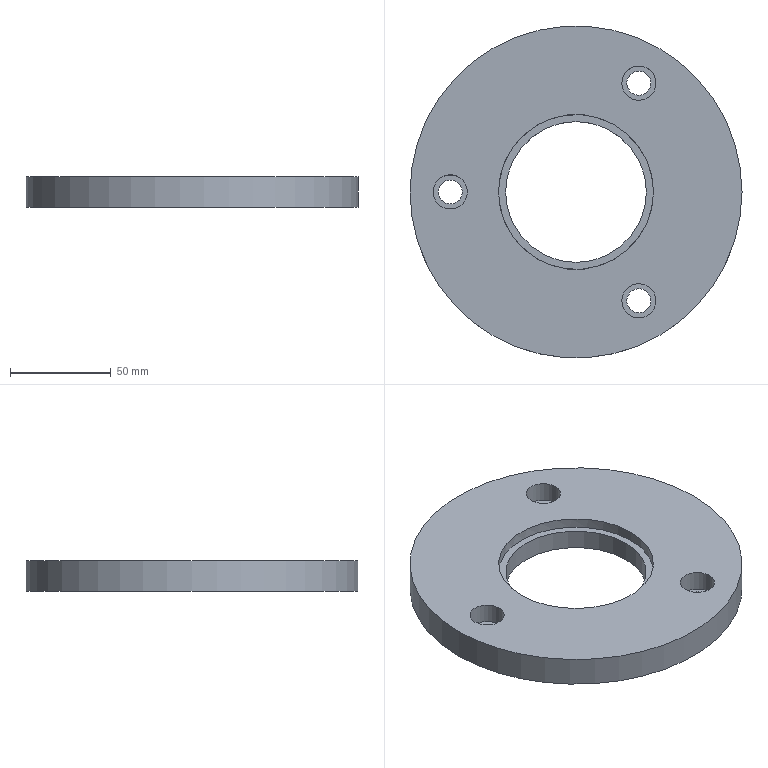Part | NX | features solid 2 | 1 solid | 15 faces | box 165 x 165 x 15 mm | volume 250463 mm3 | cylinder 9 | plane 6 | commonest cylinder face diameters 12 x3 17 x3 70 x1 77 x1 165 x1
STEP:
#1=CARTESIAN_POINT('',(231.5,-370.,50.));
#2=VERTEX_POINT('',#1);
#3=CARTESIAN_POINT('',(237.5,-370.,50.));
#4=DIRECTION('',(0.,0.,-1.));
#5=DIRECTION('',(-1.,0.,0.));
#6=AXIS2_PLACEMENT_3D('',#3,#4,#5);
#7=CIRCLE('',#6,6.);
#8=EDGE_CURVE('',#2,#2,#7,.T.);
#9=ORIENTED_EDGE('',*,*,#8,.T.);
#10=EDGE_LOOP('',(#9));
#11=FACE_BOUND('',#10,.T.);
#12=CARTESIAN_POINT('',(243.5,-370.,55.));
#13=VERTEX_POINT('',#12);
#14=CARTESIAN_POINT('',(237.5,-370.,55.));
#15=DIRECTION('',(0.,0.,1.));
#16=DIRECTION('',(1.,0.,0.));
#17=AXIS2_PLACEMENT_3D('',#14,#15,#16);
#18=CIRCLE('',#17,6.);
#19=EDGE_CURVE('',#13,#13,#18,.F.);
#20=ORIENTED_EDGE('',*,*,#19,.F.);
#21=EDGE_LOOP('',(#20));
#22=FACE_BOUND('',#21,.T.);
#23=CARTESIAN_POINT('',(237.5,-370.,45.));
#24=DIRECTION('',(0.,0.,1.));
#25=DIRECTION('',(1.,0.,0.));
#26=AXIS2_PLACEMENT_3D('',#23,#24,#25);
#27=CYLINDRICAL_SURFACE('',#26,6.);
#28=ADVANCED_FACE('',(#11,#22),#27,.F.);
#29=CARTESIAN_POINT('',(325.25,-315.873,50.));
#30=VERTEX_POINT('',#29);
#31=CARTESIAN_POINT('',(331.25,-315.873,50.));
#32=DIRECTION('',(0.,0.,-1.));
#33=DIRECTION('',(-1.,0.,0.));
#34=AXIS2_PLACEMENT_3D('',#31,#32,#33);
#35=CIRCLE('',#34,6.);
#36=EDGE_CURVE('',#30,#30,#35,.T.);
#37=ORIENTED_EDGE('',*,*,#36,.T.);
#38=EDGE_LOOP('',(#37));
#39=FACE_BOUND('',#38,.T.);
#40=CARTESIAN_POINT('',(337.25,-315.873,55.));
#41=VERTEX_POINT('',#40);
#42=CARTESIAN_POINT('',(331.25,-315.873,55.));
#43=DIRECTION('',(0.,0.,1.));
#44=DIRECTION('',(1.,0.,0.));
#45=AXIS2_PLACEMENT_3D('',#42,#43,#44);
#46=CIRCLE('',#45,6.);
#47=EDGE_CURVE('',#41,#41,#46,.F.);
#48=ORIENTED_EDGE('',*,*,#47,.F.);
#49=EDGE_LOOP('',(#48));
#50=FACE_BOUND('',#49,.T.);
#51=CARTESIAN_POINT('',(331.25,-315.873,45.));
#52=DIRECTION('',(0.,0.,1.));
#53=DIRECTION('',(1.,0.,0.));
#54=AXIS2_PLACEMENT_3D('',#51,#52,#53);
#55=CYLINDRICAL_SURFACE('',#54,6.);
#56=ADVANCED_FACE('',(#39,#50),#55,.F.);
#57=CARTESIAN_POINT('',(325.25,-424.127,50.));
#58=VERTEX_POINT('',#57);
#59=CARTESIAN_POINT('',(331.25,-424.127,50.));
#60=DIRECTION('',(0.,0.,-1.));
#61=DIRECTION('',(-1.,0.,0.));
#62=AXIS2_PLACEMENT_3D('',#59,#60,#61);
#63=CIRCLE('',#62,6.);
#64=EDGE_CURVE('',#58,#58,#63,.T.);
#65=ORIENTED_EDGE('',*,*,#64,.T.);
#66=EDGE_LOOP('',(#65));
#67=FACE_BOUND('',#66,.T.);
#68=CARTESIAN_POINT('',(337.25,-424.127,55.));
#69=VERTEX_POINT('',#68);
#70=CARTESIAN_POINT('',(331.25,-424.127,55.));
#71=DIRECTION('',(0.,0.,1.));
#72=DIRECTION('',(1.,0.,0.));
#73=AXIS2_PLACEMENT_3D('',#70,#71,#72);
#74=CIRCLE('',#73,6.);
#75=EDGE_CURVE('',#69,#69,#74,.F.);
#76=ORIENTED_EDGE('',*,*,#75,.F.);
#77=EDGE_LOOP('',(#76));
#78=FACE_BOUND('',#77,.T.);
#79=CARTESIAN_POINT('',(331.25,-424.127,45.));
#80=DIRECTION('',(0.,0.,1.));
#81=DIRECTION('',(1.,0.,0.));
#82=AXIS2_PLACEMENT_3D('',#79,#80,#81);
#83=CYLINDRICAL_SURFACE('',#82,6.);
#84=ADVANCED_FACE('',(#67,#78),#83,.F.);
#85=ORIENTED_EDGE('',*,*,#8,.F.);
#86=EDGE_LOOP('',(#85));
#87=FACE_BOUND('',#86,.T.);
#88=ORIENTED_EDGE('',*,*,#64,.F.);
#89=EDGE_LOOP('',(#88));
#90=FACE_BOUND('',#89,.T.);
#91=ORIENTED_EDGE('',*,*,#36,.F.);
#92=EDGE_LOOP('',(#91));
#93=FACE_BOUND('',#92,.T.);
#94=CARTESIAN_POINT('',(217.5,-370.,50.));
#95=VERTEX_POINT('',#94);
#96=CARTESIAN_POINT('',(300.,-370.,50.));
#97=DIRECTION('',(0.,0.,-1.));
#98=DIRECTION('',(-1.,0.,0.));
#99=AXIS2_PLACEMENT_3D('',#96,#97,#98);
#100=CIRCLE('',#99,82.5);
#101=EDGE_CURVE('',#95,#95,#100,.T.);
#102=ORIENTED_EDGE('',*,*,#101,.T.);
#103=EDGE_LOOP('',(#102));
#104=FACE_BOUND('',#103,.T.);
#105=CARTESIAN_POINT('',(265.,-370.,50.));
#106=VERTEX_POINT('',#105);
#107=CARTESIAN_POINT('',(300.,-370.,50.));
#108=DIRECTION('',(0.,0.,-1.));
#109=DIRECTION('',(-1.,0.,0.));
#110=AXIS2_PLACEMENT_3D('',#107,#108,#109);
#111=CIRCLE('',#110,35.);
#112=EDGE_CURVE('',#106,#106,#111,.F.);
#113=ORIENTED_EDGE('',*,*,#112,.T.);
#114=EDGE_LOOP('',(#113));
#115=FACE_BOUND('',#114,.T.);
#116=CARTESIAN_POINT('',(300.,-370.,50.));
#117=DIRECTION('',(0.,0.,-1.));
#118=DIRECTION('',(-1.,0.,0.));
#119=AXIS2_PLACEMENT_3D('',#116,#117,#118);
#120=PLANE('',#119);
#121=ADVANCED_FACE('',(#87,#90,#93,#104,#115),#120,.T.);
#122=CARTESIAN_POINT('',(246.,-370.,65.));
#123=VERTEX_POINT('',#122);
#124=CARTESIAN_POINT('',(237.5,-370.,65.));
#125=DIRECTION('',(0.,0.,1.));
#126=DIRECTION('',(1.,0.,0.));
#127=AXIS2_PLACEMENT_3D('',#124,#125,#126);
#128=CIRCLE('',#127,8.5);
#129=EDGE_CURVE('',#123,#123,#128,.T.);
#130=ORIENTED_EDGE('',*,*,#129,.F.);
#131=EDGE_LOOP('',(#130));
#132=FACE_BOUND('',#131,.T.);
#133=CARTESIAN_POINT('',(339.75,-315.873,65.));
#134=VERTEX_POINT('',#133);
#135=CARTESIAN_POINT('',(331.25,-315.873,65.));
#136=DIRECTION('',(0.,0.,1.));
#137=DIRECTION('',(1.,0.,0.));
#138=AXIS2_PLACEMENT_3D('',#135,#136,#137);
#139=CIRCLE('',#138,8.5);
#140=EDGE_CURVE('',#134,#134,#139,.T.);
#141=ORIENTED_EDGE('',*,*,#140,.F.);
#142=EDGE_LOOP('',(#141));
#143=FACE_BOUND('',#142,.T.);
#144=CARTESIAN_POINT('',(339.75,-424.127,65.));
#145=VERTEX_POINT('',#144);
#146=CARTESIAN_POINT('',(331.25,-424.127,65.));
#147=DIRECTION('',(0.,0.,1.));
#148=DIRECTION('',(1.,0.,0.));
#149=AXIS2_PLACEMENT_3D('',#146,#147,#148);
#150=CIRCLE('',#149,8.5);
#151=EDGE_CURVE('',#145,#145,#150,.T.);
#152=ORIENTED_EDGE('',*,*,#151,.F.);
#153=EDGE_LOOP('',(#152));
#154=FACE_BOUND('',#153,.T.);
#155=CARTESIAN_POINT('',(217.5,-370.,65.));
#156=VERTEX_POINT('',#155);
#157=CARTESIAN_POINT('',(300.,-370.,65.));
#158=DIRECTION('',(0.,0.,-1.));
#159=DIRECTION('',(-1.,0.,0.));
#160=AXIS2_PLACEMENT_3D('',#157,#158,#159);
#161=CIRCLE('',#160,82.5);
#162=EDGE_CURVE('',#156,#156,#161,.T.);
#163=ORIENTED_EDGE('',*,*,#162,.F.);
#164=EDGE_LOOP('',(#163));
#165=FACE_BOUND('',#164,.T.);
#166=CARTESIAN_POINT('',(261.5,-370.,65.));
#167=VERTEX_POINT('',#166);
#168=CARTESIAN_POINT('',(300.,-370.,65.));
#169=DIRECTION('',(0.,0.,-1.));
#170=DIRECTION('',(-1.,0.,0.));
#171=AXIS2_PLACEMENT_3D('',#168,#169,#170);
#172=CIRCLE('',#171,38.5);
#173=EDGE_CURVE('',#167,#167,#172,.T.);
#174=ORIENTED_EDGE('',*,*,#173,.T.);
#175=EDGE_LOOP('',(#174));
#176=FACE_BOUND('',#175,.T.);
#177=CARTESIAN_POINT('',(300.,-370.,65.));
#178=DIRECTION('',(0.,0.,-1.));
#179=DIRECTION('',(-1.,0.,0.));
#180=AXIS2_PLACEMENT_3D('',#177,#178,#179);
#181=PLANE('',#180);
#182=ADVANCED_FACE('',(#132,#143,#154,#165,#176),#181,.F.);
#183=ORIENTED_EDGE('',*,*,#101,.F.);
#184=EDGE_LOOP('',(#183));
#185=FACE_BOUND('',#184,.T.);
#186=ORIENTED_EDGE('',*,*,#162,.T.);
#187=EDGE_LOOP('',(#186));
#188=FACE_BOUND('',#187,.T.);
#189=CARTESIAN_POINT('',(300.,-370.,50.));
#190=DIRECTION('',(0.,0.,1.));
#191=DIRECTION('',(1.,0.,0.));
#192=AXIS2_PLACEMENT_3D('',#189,#190,#191);
#193=CYLINDRICAL_SURFACE('',#192,82.5);
#194=ADVANCED_FACE('',(#185,#188),#193,.T.);
#195=ORIENTED_EDGE('',*,*,#112,.F.);
#196=EDGE_LOOP('',(#195));
#197=FACE_BOUND('',#196,.T.);
#198=CARTESIAN_POINT('',(335.,-370.,60.));
#199=VERTEX_POINT('',#198);
#200=CARTESIAN_POINT('',(300.,-370.,60.));
#201=DIRECTION('',(0.,0.,1.));
#202=DIRECTION('',(1.,0.,0.));
#203=AXIS2_PLACEMENT_3D('',#200,#201,#202);
#204=CIRCLE('',#203,35.);
#205=EDGE_CURVE('',#199,#199,#204,.F.);
#206=ORIENTED_EDGE('',*,*,#205,.F.);
#207=EDGE_LOOP('',(#206));
#208=FACE_BOUND('',#207,.T.);
#209=CARTESIAN_POINT('',(300.,-370.,-10.));
#210=DIRECTION('',(0.,0.,1.));
#211=DIRECTION('',(1.,0.,0.));
#212=AXIS2_PLACEMENT_3D('',#209,#210,#211);
#213=CYLINDRICAL_SURFACE('',#212,35.);
#214=ADVANCED_FACE('',(#197,#208),#213,.F.);
#215=ORIENTED_EDGE('',*,*,#173,.F.);
#216=EDGE_LOOP('',(#215));
#217=FACE_BOUND('',#216,.T.);
#218=CARTESIAN_POINT('',(338.5,-370.,60.));
#219=VERTEX_POINT('',#218);
#220=CARTESIAN_POINT('',(300.,-370.,60.));
#221=DIRECTION('',(0.,0.,1.));
#222=DIRECTION('',(1.,0.,0.));
#223=AXIS2_PLACEMENT_3D('',#220,#221,#222);
#224=CIRCLE('',#223,38.5);
#225=EDGE_CURVE('',#219,#219,#224,.F.);
#226=ORIENTED_EDGE('',*,*,#225,.T.);
#227=EDGE_LOOP('',(#226));
#228=FACE_BOUND('',#227,.T.);
#229=CARTESIAN_POINT('',(300.,-370.,55.));
#230=DIRECTION('',(0.,0.,1.));
#231=DIRECTION('',(1.,0.,0.));
#232=AXIS2_PLACEMENT_3D('',#229,#230,#231);
#233=CYLINDRICAL_SURFACE('',#232,38.5);
#234=ADVANCED_FACE('',(#217,#228),#233,.F.);
#235=ORIENTED_EDGE('',*,*,#225,.F.);
#236=EDGE_LOOP('',(#235));
#237=FACE_BOUND('',#236,.T.);
#238=ORIENTED_EDGE('',*,*,#205,.T.);
#239=EDGE_LOOP('',(#238));
#240=FACE_BOUND('',#239,.T.);
#241=CARTESIAN_POINT('',(300.,-370.,60.));
#242=DIRECTION('',(0.,0.,1.));
#243=DIRECTION('',(1.,0.,0.));
#244=AXIS2_PLACEMENT_3D('',#241,#242,#243);
#245=PLANE('',#244);
#246=ADVANCED_FACE('',(#237,#240),#245,.T.);
#247=CARTESIAN_POINT('',(339.75,-424.127,55.));
#248=VERTEX_POINT('',#247);
#249=CARTESIAN_POINT('',(331.25,-424.127,55.));
#250=DIRECTION('',(0.,0.,1.));
#251=DIRECTION('',(1.,0.,0.));
#252=AXIS2_PLACEMENT_3D('',#249,#250,#251);
#253=CIRCLE('',#252,8.5);
#254=EDGE_CURVE('',#248,#248,#253,.T.);
#255=ORIENTED_EDGE('',*,*,#254,.T.);
#256=EDGE_LOOP('',(#255));
#257=FACE_BOUND('',#256,.T.);
#258=ORIENTED_EDGE('',*,*,#75,.T.);
#259=EDGE_LOOP('',(#258));
#260=FACE_BOUND('',#259,.T.);
#261=CARTESIAN_POINT('',(331.25,-424.127,55.));
#262=DIRECTION('',(0.,0.,1.));
#263=DIRECTION('',(1.,0.,0.));
#264=AXIS2_PLACEMENT_3D('',#261,#262,#263);
#265=PLANE('',#264);
#266=ADVANCED_FACE('',(#257,#260),#265,.T.);
#267=ORIENTED_EDGE('',*,*,#254,.F.);
#268=EDGE_LOOP('',(#267));
#269=FACE_BOUND('',#268,.T.);
#270=ORIENTED_EDGE('',*,*,#151,.T.);
#271=EDGE_LOOP('',(#270));
#272=FACE_BOUND('',#271,.T.);
#273=CARTESIAN_POINT('',(331.25,-424.127,55.));
#274=DIRECTION('',(0.,0.,1.));
#275=DIRECTION('',(1.,0.,0.));
#276=AXIS2_PLACEMENT_3D('',#273,#274,#275);
#277=CYLINDRICAL_SURFACE('',#276,8.5);
#278=ADVANCED_FACE('',(#269,#272),#277,.F.);
#279=CARTESIAN_POINT('',(339.75,-315.873,55.));
#280=VERTEX_POINT('',#279);
#281=CARTESIAN_POINT('',(331.25,-315.873,55.));
#282=DIRECTION('',(0.,0.,1.));
#283=DIRECTION('',(1.,0.,0.));
#284=AXIS2_PLACEMENT_3D('',#281,#282,#283);
#285=CIRCLE('',#284,8.5);
#286=EDGE_CURVE('',#280,#280,#285,.T.);
#287=ORIENTED_EDGE('',*,*,#286,.T.);
#288=EDGE_LOOP('',(#287));
#289=FACE_BOUND('',#288,.T.);
#290=ORIENTED_EDGE('',*,*,#47,.T.);
#291=EDGE_LOOP('',(#290));
#292=FACE_BOUND('',#291,.T.);
#293=CARTESIAN_POINT('',(331.25,-315.873,55.));
#294=DIRECTION('',(0.,0.,1.));
#295=DIRECTION('',(1.,0.,0.));
#296=AXIS2_PLACEMENT_3D('',#293,#294,#295);
#297=PLANE('',#296);
#298=ADVANCED_FACE('',(#289,#292),#297,.T.);
#299=ORIENTED_EDGE('',*,*,#286,.F.);
#300=EDGE_LOOP('',(#299));
#301=FACE_BOUND('',#300,.T.);
#302=ORIENTED_EDGE('',*,*,#140,.T.);
#303=EDGE_LOOP('',(#302));
#304=FACE_BOUND('',#303,.T.);
#305=CARTESIAN_POINT('',(331.25,-315.873,55.));
#306=DIRECTION('',(0.,0.,1.));
#307=DIRECTION('',(1.,0.,0.));
#308=AXIS2_PLACEMENT_3D('',#305,#306,#307);
#309=CYLINDRICAL_SURFACE('',#308,8.5);
#310=ADVANCED_FACE('',(#301,#304),#309,.F.);
#311=CARTESIAN_POINT('',(246.,-370.,55.));
#312=VERTEX_POINT('',#311);
#313=CARTESIAN_POINT('',(237.5,-370.,55.));
#314=DIRECTION('',(0.,0.,1.));
#315=DIRECTION('',(1.,0.,0.));
#316=AXIS2_PLACEMENT_3D('',#313,#314,#315);
#317=CIRCLE('',#316,8.5);
#318=EDGE_CURVE('',#312,#312,#317,.T.);
#319=ORIENTED_EDGE('',*,*,#318,.T.);
#320=EDGE_LOOP('',(#319));
#321=FACE_BOUND('',#320,.T.);
#322=ORIENTED_EDGE('',*,*,#19,.T.);
#323=EDGE_LOOP('',(#322));
#324=FACE_BOUND('',#323,.T.);
#325=CARTESIAN_POINT('',(237.5,-370.,55.));
#326=DIRECTION('',(0.,0.,1.));
#327=DIRECTION('',(1.,0.,0.));
#328=AXIS2_PLACEMENT_3D('',#325,#326,#327);
#329=PLANE('',#328);
#330=ADVANCED_FACE('',(#321,#324),#329,.T.);
#331=ORIENTED_EDGE('',*,*,#318,.F.);
#332=EDGE_LOOP('',(#331));
#333=FACE_BOUND('',#332,.T.);
#334=ORIENTED_EDGE('',*,*,#129,.T.);
#335=EDGE_LOOP('',(#334));
#336=FACE_BOUND('',#335,.T.);
#337=CARTESIAN_POINT('',(237.5,-370.,55.));
#338=DIRECTION('',(0.,0.,1.));
#339=DIRECTION('',(1.,0.,0.));
#340=AXIS2_PLACEMENT_3D('',#337,#338,#339);
#341=CYLINDRICAL_SURFACE('',#340,8.5);
#342=ADVANCED_FACE('',(#333,#336),#341,.F.);
#343=CLOSED_SHELL('',(#28,#56,#84,#121,#182,#194,#214,#234,#246,#266,#278,#298,#310,#330,#342));
#344=MANIFOLD_SOLID_BREP('',#343);
#345=(LENGTH_UNIT()NAMED_UNIT(*)SI_UNIT(.MILLI.,.METRE.));
#346=UNCERTAINTY_MEASURE_WITH_UNIT(LENGTH_MEASURE(0.00001),#345,'','');
#347=(NAMED_UNIT(*)PLANE_ANGLE_UNIT()SI_UNIT($,.RADIAN.));
#348=(NAMED_UNIT(*)SI_UNIT($,.STERADIAN.)SOLID_ANGLE_UNIT());
#349=(GEOMETRIC_REPRESENTATION_CONTEXT(3)GLOBAL_UNCERTAINTY_ASSIGNED_CONTEXT((#346))GLOBAL_UNIT_ASSIGNED_CONTEXT((#345,#347,#348))REPRESENTATION_CONTEXT('',''));
#350=ADVANCED_BREP_SHAPE_REPRESENTATION('',(#344),#349);